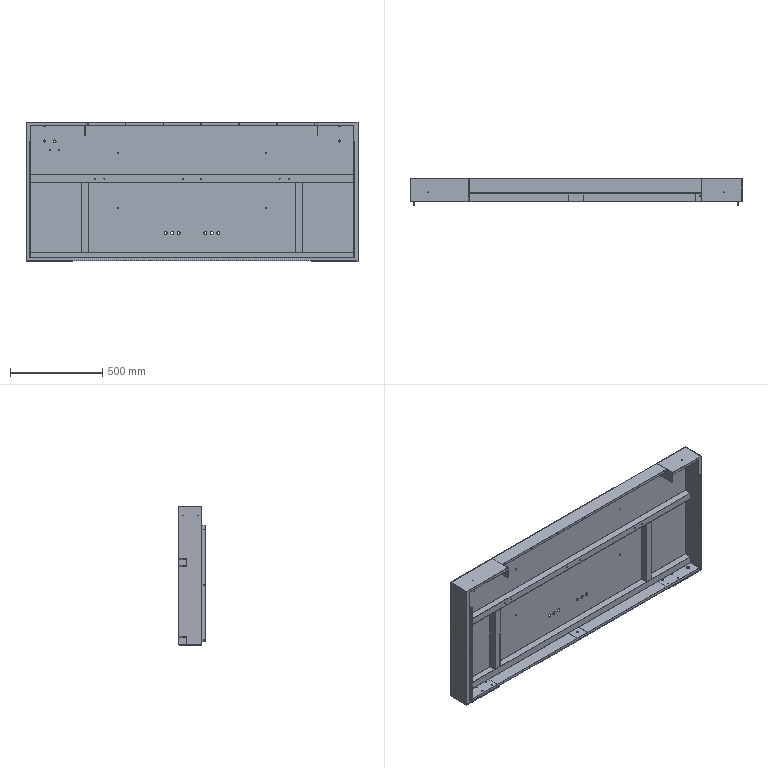Part | STEP file | 9 solids | 244 faces | box 1800 x 145 x 755 mm | volume 5256962 mm3 | cylinder 140 | plane 100 | cone 4 | commonest cylinder face diameters 6.8 x40 4.2 x24 12 x18 3.4 x14 16 x14 5.2 x12